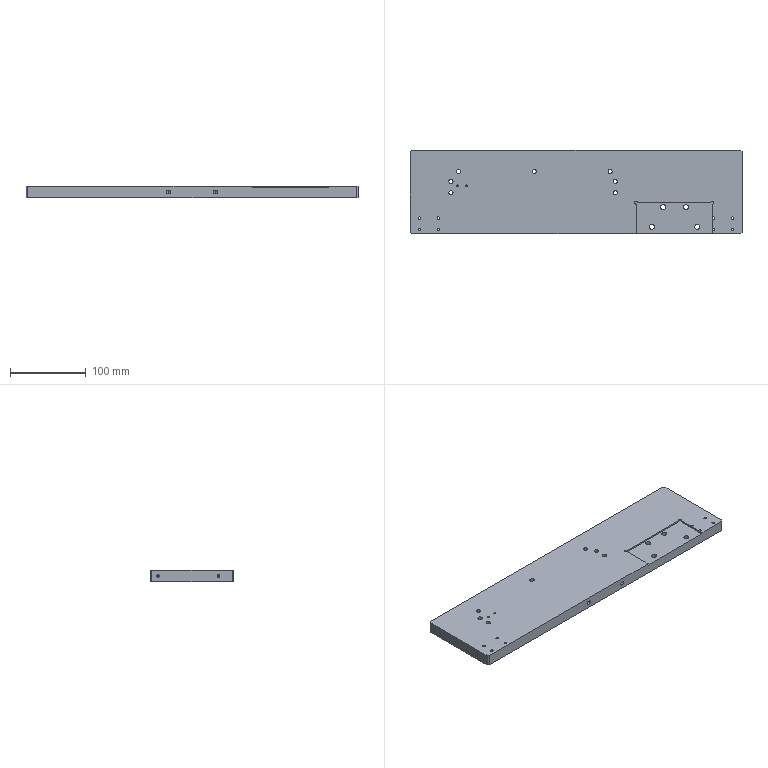Part | STEP file | FBDS-CS-031 | 1 solid | 142 faces | box 438 x 110 x 15 mm | volume 703855 mm3 | cylinder 87 | cone 28 | plane 27 | commonest cylinder face diameters 3.3 x28 5.5 x14 10 x14 2.5 x8 6.6 x8 11 x8